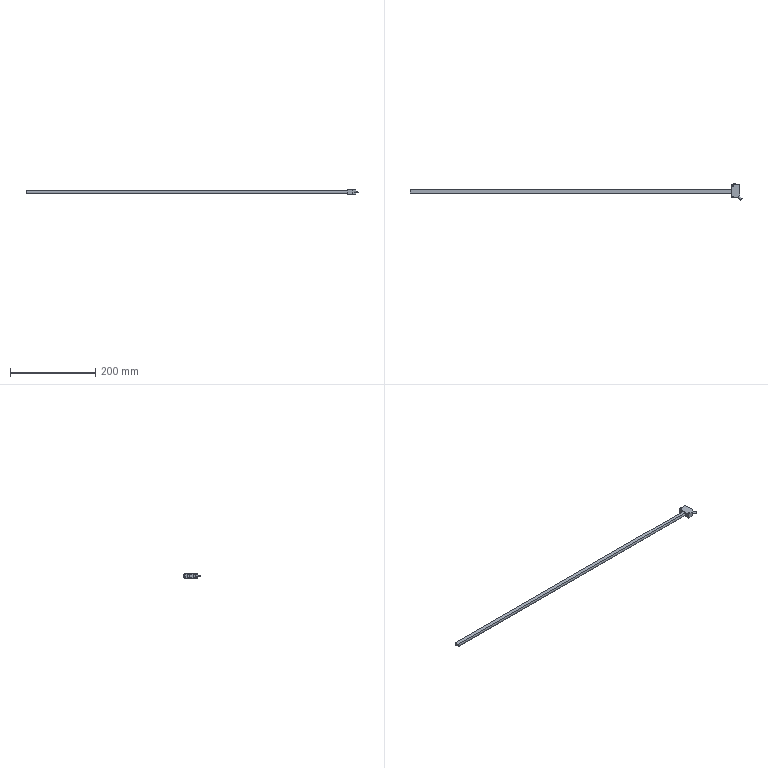Part | SolidWorks | features BaseBody 1, ICE 1 | 1 solid | 66 faces | box 779.985 x 38.085 x 10.8 mm | volume 59248 mm3 | plane 49 | cylinder 17 | commonest cylinder face diameters 2.6 x4 3 x4 4.5 x3 4 x2 10.8 x2 11 x2